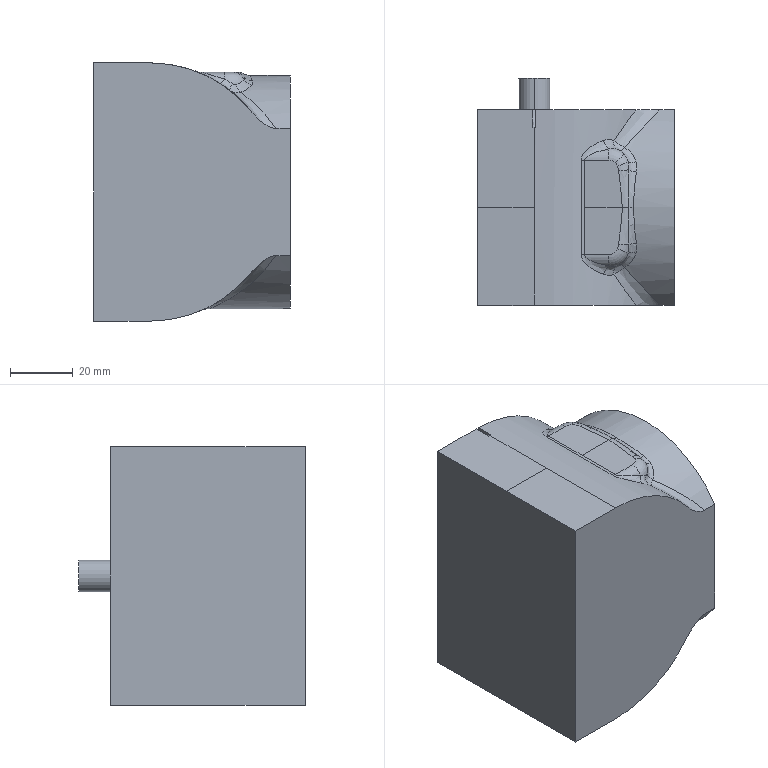Part | STEP file | ASND-0110-IRB120_3-58_IRC5_Link5_rev0-2 | 1 solid | 46 faces | box 62.5 x 72 x 82 mm | volume 291195 mm3 | spline 20 | plane 13 | cylinder 10 | other 3 | commonest cylinder face diameters 8 x2 10 x2 74 x2 82 x2 6 x1 40 x1